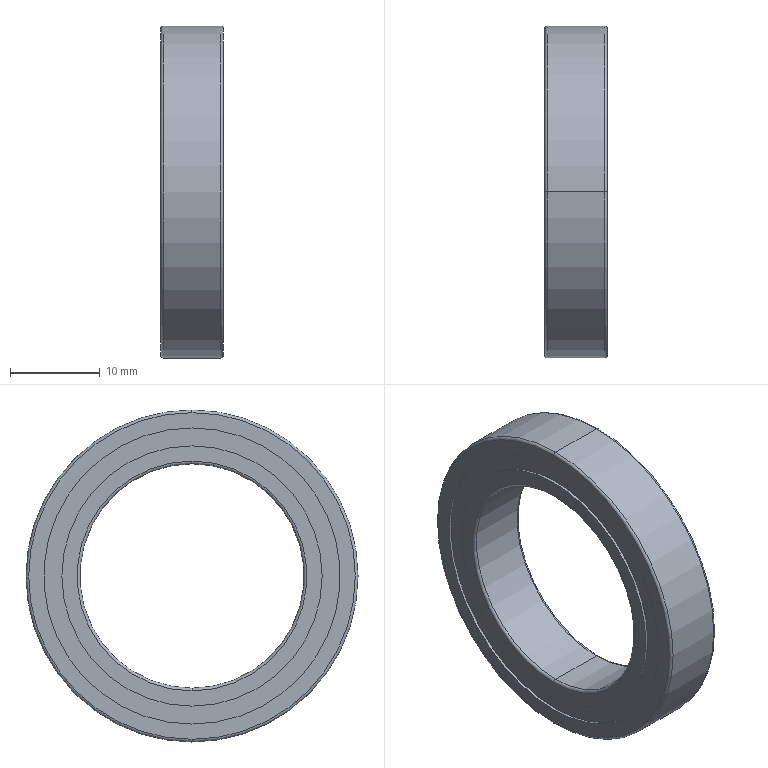Part | STEP file | 61805ZZ_Rolling bearings 61805 GB 276-94 | 1 solid | 194 faces | box 7 x 37 x 37 mm | volume 3206 mm3 | torus 104 | sphere 62 | cylinder 20 | plane 8 | commonest cylinder face diameters 29 x8 33 x8 25 x2 37 x2